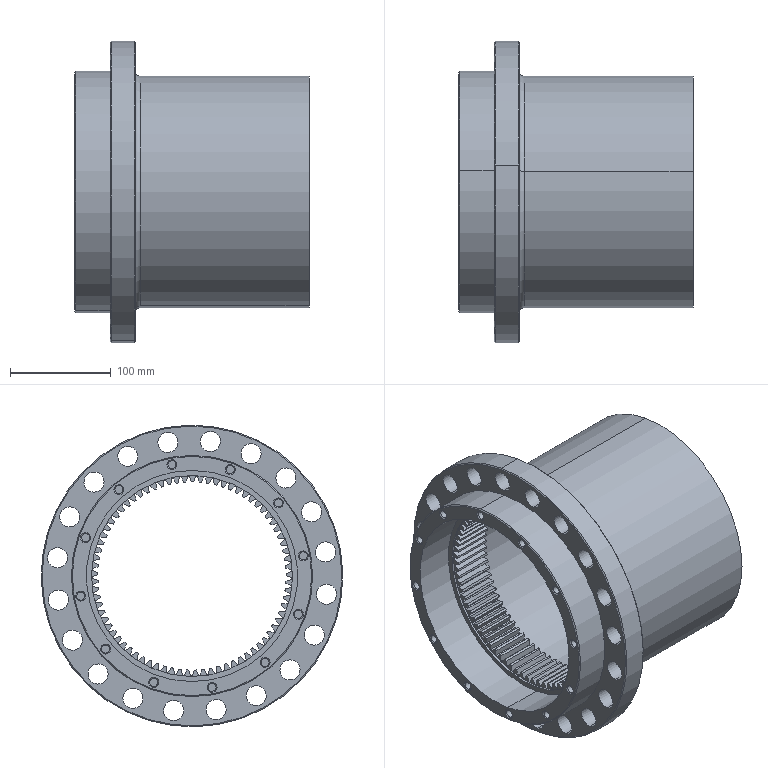Part | NX | features BREP 1 | 1 solid | 450 faces | box 233 x 300 x 300 mm | volume 2767073 mm3 | cylinder 240 | spline 154 | cone 30 | plane 24 | torus 2 | commonest cylinder face diameters 187.195 x77 198.75 x77 20 x40 8 x24 210 x8 200 x4